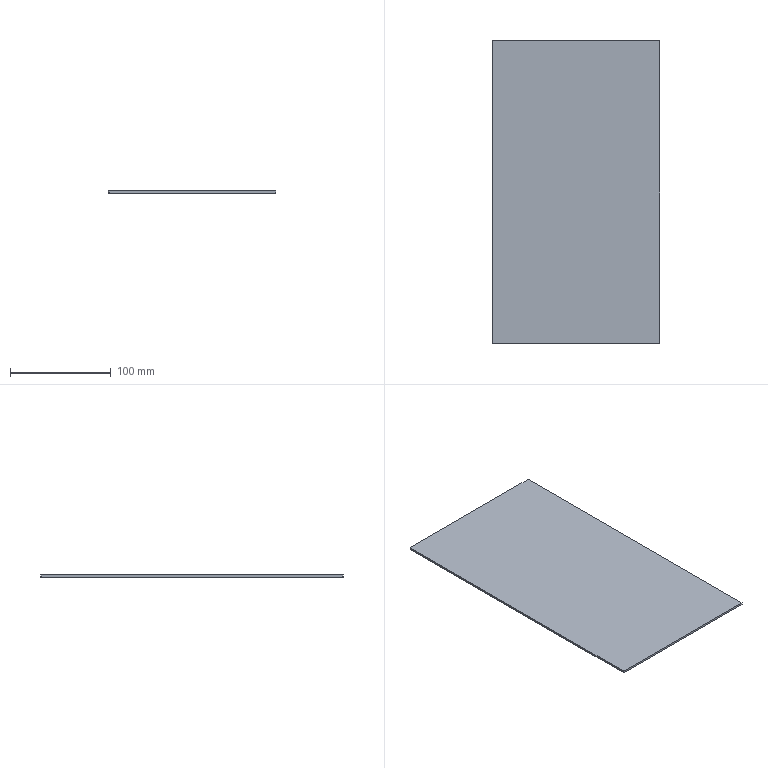Part | STEP file | Oil Filler Tank Closing Plate 1 | 1 solid | 8 faces | box 166.5 x 301 x 2 mm | volume 100233 mm3 | plane 6 | cylinder 2 | commonest cylinder face diameters 1.5 x2
STEP:
#1=CARTESIAN_POINT('',(-168.5,-149.75,-2.));
#2=VERTEX_POINT('',#1);
#3=CARTESIAN_POINT('',(-167.75,-150.5,-2.));
#4=VERTEX_POINT('',#3);
#5=CARTESIAN_POINT('',(-167.75,-149.75,-2.));
#6=DIRECTION('',(0.,0.,1.));
#7=DIRECTION('',(1.,0.,0.));
#8=AXIS2_PLACEMENT_3D('',#5,#6,#7);
#9=CIRCLE('',#8,0.75);
#10=EDGE_CURVE('',#2,#4,#9,.T.);
#11=ORIENTED_EDGE('',*,*,#10,.F.);
#12=CARTESIAN_POINT('',(-168.5,149.75,-2.));
#13=VERTEX_POINT('',#12);
#14=CARTESIAN_POINT('',(-168.5,0.,-2.));
#15=DIRECTION('',(0.,-1.,0.));
#16=VECTOR('',#15,1000.);
#17=LINE('',#14,#16);
#18=EDGE_CURVE('',#13,#2,#17,.T.);
#19=ORIENTED_EDGE('',*,*,#18,.F.);
#20=CARTESIAN_POINT('',(-167.75,150.5,-2.));
#21=VERTEX_POINT('',#20);
#22=CARTESIAN_POINT('',(-167.75,149.75,-2.));
#23=DIRECTION('',(0.,0.,1.));
#24=DIRECTION('',(1.,0.,0.));
#25=AXIS2_PLACEMENT_3D('',#22,#23,#24);
#26=CIRCLE('',#25,0.75);
#27=EDGE_CURVE('',#21,#13,#26,.T.);
#28=ORIENTED_EDGE('',*,*,#27,.F.);
#29=CARTESIAN_POINT('',(-2.,150.5,-2.));
#30=VERTEX_POINT('',#29);
#31=CARTESIAN_POINT('',(0.,150.5,-2.));
#32=DIRECTION('',(-1.,0.,0.));
#33=VECTOR('',#32,1000.);
#34=LINE('',#31,#33);
#35=EDGE_CURVE('',#30,#21,#34,.T.);
#36=ORIENTED_EDGE('',*,*,#35,.F.);
#37=CARTESIAN_POINT('',(-2.,-150.5,-2.));
#38=VERTEX_POINT('',#37);
#39=CARTESIAN_POINT('',(-2.,0.,-2.));
#40=DIRECTION('',(0.,1.,0.));
#41=VECTOR('',#40,1000.);
#42=LINE('',#39,#41);
#43=EDGE_CURVE('',#38,#30,#42,.T.);
#44=ORIENTED_EDGE('',*,*,#43,.F.);
#45=CARTESIAN_POINT('',(0.,-150.5,-2.));
#46=DIRECTION('',(1.,0.,0.));
#47=VECTOR('',#46,1000.);
#48=LINE('',#45,#47);
#49=EDGE_CURVE('',#4,#38,#48,.T.);
#50=ORIENTED_EDGE('',*,*,#49,.F.);
#51=EDGE_LOOP('',(#11,#19,#28,#36,#44,#50));
#52=FACE_OUTER_BOUND('',#51,.T.);
#53=CARTESIAN_POINT('',(0.,0.,-2.));
#54=DIRECTION('',(0.,0.,1.));
#55=DIRECTION('',(1.,0.,0.));
#56=AXIS2_PLACEMENT_3D('',#53,#54,#55);
#57=PLANE('',#56);
#58=ADVANCED_FACE('',(#52),#57,.F.);
#59=ORIENTED_EDGE('',*,*,#49,.T.);
#60=CARTESIAN_POINT('',(-2.,-150.5,0.));
#61=VERTEX_POINT('',#60);
#62=CARTESIAN_POINT('',(-2.,-150.5,-2.));
#63=DIRECTION('',(0.,0.,1.));
#64=VECTOR('',#63,1000.);
#65=LINE('',#62,#64);
#66=EDGE_CURVE('',#38,#61,#65,.T.);
#67=ORIENTED_EDGE('',*,*,#66,.T.);
#68=CARTESIAN_POINT('',(-167.75,-150.5,0.));
#69=VERTEX_POINT('',#68);
#70=CARTESIAN_POINT('',(-168.5,-150.5,0.));
#71=DIRECTION('',(-1.,0.,0.));
#72=VECTOR('',#71,1000.);
#73=LINE('',#70,#72);
#74=EDGE_CURVE('',#61,#69,#73,.T.);
#75=ORIENTED_EDGE('',*,*,#74,.T.);
#76=CARTESIAN_POINT('',(-167.75,-150.5,-2.));
#77=DIRECTION('',(0.,0.,-1.));
#78=VECTOR('',#77,1000.);
#79=LINE('',#76,#78);
#80=EDGE_CURVE('',#69,#4,#79,.T.);
#81=ORIENTED_EDGE('',*,*,#80,.T.);
#82=EDGE_LOOP('',(#59,#67,#75,#81));
#83=FACE_OUTER_BOUND('',#82,.T.);
#84=CARTESIAN_POINT('',(-168.5,-150.5,-2.));
#85=DIRECTION('',(0.,-1.,0.));
#86=DIRECTION('',(0.,0.,-1.));
#87=AXIS2_PLACEMENT_3D('',#84,#85,#86);
#88=PLANE('',#87);
#89=ADVANCED_FACE('',(#83),#88,.T.);
#90=CARTESIAN_POINT('',(-168.5,-149.75,0.));
#91=VERTEX_POINT('',#90);
#92=CARTESIAN_POINT('',(-168.5,149.75,0.));
#93=VERTEX_POINT('',#92);
#94=CARTESIAN_POINT('',(-168.5,150.5,0.));
#95=DIRECTION('',(0.,1.,0.));
#96=VECTOR('',#95,1000.);
#97=LINE('',#94,#96);
#98=EDGE_CURVE('',#91,#93,#97,.T.);
#99=ORIENTED_EDGE('',*,*,#98,.T.);
#100=CARTESIAN_POINT('',(-168.5,149.75,-2.));
#101=DIRECTION('',(0.,0.,-1.));
#102=VECTOR('',#101,1000.);
#103=LINE('',#100,#102);
#104=EDGE_CURVE('',#93,#13,#103,.T.);
#105=ORIENTED_EDGE('',*,*,#104,.T.);
#106=ORIENTED_EDGE('',*,*,#18,.T.);
#107=CARTESIAN_POINT('',(-168.5,-149.75,-2.));
#108=DIRECTION('',(0.,0.,1.));
#109=VECTOR('',#108,1000.);
#110=LINE('',#107,#109);
#111=EDGE_CURVE('',#2,#91,#110,.T.);
#112=ORIENTED_EDGE('',*,*,#111,.T.);
#113=EDGE_LOOP('',(#99,#105,#106,#112));
#114=FACE_OUTER_BOUND('',#113,.T.);
#115=CARTESIAN_POINT('',(-168.5,150.5,-2.));
#116=DIRECTION('',(-1.,0.,0.));
#117=DIRECTION('',(0.,0.,1.));
#118=AXIS2_PLACEMENT_3D('',#115,#116,#117);
#119=PLANE('',#118);
#120=ADVANCED_FACE('',(#114),#119,.T.);
#121=CARTESIAN_POINT('',(-167.75,150.5,0.));
#122=VERTEX_POINT('',#121);
#123=CARTESIAN_POINT('',(-2.,150.5,0.));
#124=VERTEX_POINT('',#123);
#125=CARTESIAN_POINT('',(-168.5,150.5,0.));
#126=DIRECTION('',(1.,0.,0.));
#127=VECTOR('',#126,1000.);
#128=LINE('',#125,#127);
#129=EDGE_CURVE('',#122,#124,#128,.T.);
#130=ORIENTED_EDGE('',*,*,#129,.T.);
#131=CARTESIAN_POINT('',(-2.,150.5,-2.));
#132=DIRECTION('',(0.,0.,-1.));
#133=VECTOR('',#132,1000.);
#134=LINE('',#131,#133);
#135=EDGE_CURVE('',#124,#30,#134,.T.);
#136=ORIENTED_EDGE('',*,*,#135,.T.);
#137=ORIENTED_EDGE('',*,*,#35,.T.);
#138=CARTESIAN_POINT('',(-167.75,150.5,-2.));
#139=DIRECTION('',(0.,0.,1.));
#140=VECTOR('',#139,1000.);
#141=LINE('',#138,#140);
#142=EDGE_CURVE('',#21,#122,#141,.T.);
#143=ORIENTED_EDGE('',*,*,#142,.T.);
#144=EDGE_LOOP('',(#130,#136,#137,#143));
#145=FACE_OUTER_BOUND('',#144,.T.);
#146=CARTESIAN_POINT('',(-168.5,150.5,-2.));
#147=DIRECTION('',(0.,1.,0.));
#148=DIRECTION('',(0.,0.,1.));
#149=AXIS2_PLACEMENT_3D('',#146,#147,#148);
#150=PLANE('',#149);
#151=ADVANCED_FACE('',(#145),#150,.T.);
#152=ORIENTED_EDGE('',*,*,#43,.T.);
#153=ORIENTED_EDGE('',*,*,#135,.F.);
#154=CARTESIAN_POINT('',(-2.,150.5,0.));
#155=DIRECTION('',(0.,-1.,0.));
#156=VECTOR('',#155,1000.);
#157=LINE('',#154,#156);
#158=EDGE_CURVE('',#124,#61,#157,.T.);
#159=ORIENTED_EDGE('',*,*,#158,.T.);
#160=ORIENTED_EDGE('',*,*,#66,.F.);
#161=EDGE_LOOP('',(#152,#153,#159,#160));
#162=FACE_OUTER_BOUND('',#161,.T.);
#163=CARTESIAN_POINT('',(-2.,150.5,-2.));
#164=DIRECTION('',(1.,0.,0.));
#165=DIRECTION('',(0.,0.,-1.));
#166=AXIS2_PLACEMENT_3D('',#163,#164,#165);
#167=PLANE('',#166);
#168=ADVANCED_FACE('',(#162),#167,.T.);
#169=CARTESIAN_POINT('',(-167.75,-149.75,0.));
#170=DIRECTION('',(0.,0.,-1.));
#171=DIRECTION('',(1.,0.,0.));
#172=AXIS2_PLACEMENT_3D('',#169,#170,#171);
#173=CIRCLE('',#172,0.75);
#174=EDGE_CURVE('',#69,#91,#173,.T.);
#175=ORIENTED_EDGE('',*,*,#174,.T.);
#176=ORIENTED_EDGE('',*,*,#111,.F.);
#177=ORIENTED_EDGE('',*,*,#10,.T.);
#178=ORIENTED_EDGE('',*,*,#80,.F.);
#179=EDGE_LOOP('',(#175,#176,#177,#178));
#180=FACE_OUTER_BOUND('',#179,.T.);
#181=CARTESIAN_POINT('',(-167.75,-149.75,-2.));
#182=DIRECTION('',(0.,0.,1.));
#183=DIRECTION('',(1.,0.,0.));
#184=AXIS2_PLACEMENT_3D('',#181,#182,#183);
#185=CYLINDRICAL_SURFACE('',#184,0.75);
#186=ADVANCED_FACE('',(#180),#185,.T.);
#187=ORIENTED_EDGE('',*,*,#129,.F.);
#188=CARTESIAN_POINT('',(-167.75,149.75,0.));
#189=DIRECTION('',(0.,0.,1.));
#190=DIRECTION('',(1.,0.,0.));
#191=AXIS2_PLACEMENT_3D('',#188,#189,#190);
#192=CIRCLE('',#191,0.75);
#193=EDGE_CURVE('',#122,#93,#192,.T.);
#194=ORIENTED_EDGE('',*,*,#193,.T.);
#195=ORIENTED_EDGE('',*,*,#98,.F.);
#196=ORIENTED_EDGE('',*,*,#174,.F.);
#197=ORIENTED_EDGE('',*,*,#74,.F.);
#198=ORIENTED_EDGE('',*,*,#158,.F.);
#199=EDGE_LOOP('',(#187,#194,#195,#196,#197,#198));
#200=FACE_OUTER_BOUND('',#199,.T.);
#201=CARTESIAN_POINT('',(0.,0.,0.));
#202=DIRECTION('',(0.,0.,1.));
#203=DIRECTION('',(1.,0.,0.));
#204=AXIS2_PLACEMENT_3D('',#201,#202,#203);
#205=PLANE('',#204);
#206=ADVANCED_FACE('',(#200),#205,.T.);
#207=ORIENTED_EDGE('',*,*,#193,.F.);
#208=ORIENTED_EDGE('',*,*,#142,.F.);
#209=ORIENTED_EDGE('',*,*,#27,.T.);
#210=ORIENTED_EDGE('',*,*,#104,.F.);
#211=EDGE_LOOP('',(#207,#208,#209,#210));
#212=FACE_OUTER_BOUND('',#211,.T.);
#213=CARTESIAN_POINT('',(-167.75,149.75,-2.));
#214=DIRECTION('',(0.,0.,1.));
#215=DIRECTION('',(1.,0.,0.));
#216=AXIS2_PLACEMENT_3D('',#213,#214,#215);
#217=CYLINDRICAL_SURFACE('',#216,0.75);
#218=ADVANCED_FACE('',(#212),#217,.T.);
#219=CLOSED_SHELL('',(#58,#89,#120,#151,#168,#186,#206,#218));
#220=MANIFOLD_SOLID_BREP('',#219);
#221=CARTESIAN_POINT('',(0.,0.,0.));
#222=DIRECTION('',(0.,0.,1.));
#223=DIRECTION('',(1.,0.,0.));
#224=AXIS2_PLACEMENT_3D('',#221,#222,#223);
#225=(LENGTH_UNIT()NAMED_UNIT(*)SI_UNIT(.MILLI.,.METRE.));
#226=UNCERTAINTY_MEASURE_WITH_UNIT(LENGTH_MEASURE(0.00001),#225,'','');
#227=(NAMED_UNIT(*)PLANE_ANGLE_UNIT()SI_UNIT($,.RADIAN.));
#228=(NAMED_UNIT(*)SI_UNIT($,.STERADIAN.)SOLID_ANGLE_UNIT());
#229=(GEOMETRIC_REPRESENTATION_CONTEXT(3)GLOBAL_UNCERTAINTY_ASSIGNED_CONTEXT((#226))GLOBAL_UNIT_ASSIGNED_CONTEXT((#225,#227,#228))REPRESENTATION_CONTEXT('',''));
#230=ADVANCED_BREP_SHAPE_REPRESENTATION('',(#220,#224),#229);